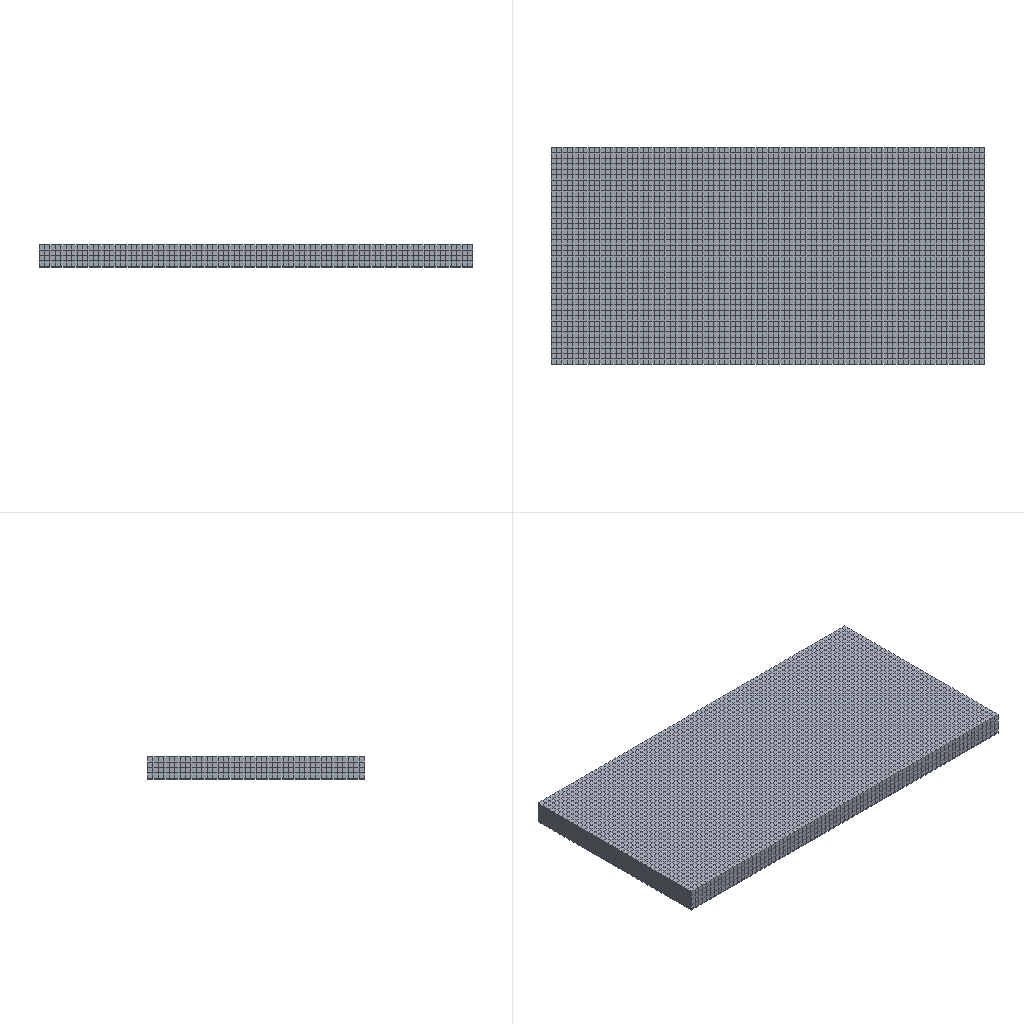Simulation study | abaqus
Set-up summary:
category,name,step,type,value,unit,region
solver,abaqus
solver,version,,,Abaqus/Explicit 2020
units,not stated in the deck,,not stated
analysis,deck,,transient,transient
load_step,Step-1,Step-1,transient
load_step,requested,,,1
mesh,nodes,,,23247
mesh,elements,,,19200
element_type,C3D8R,,solid,16000
element_type,COH3D8,,cohesive,3200
load,load commands in deck,,count,1
bc,support commands in deck,,count,1
material,BASE,,in results
material,COH,,in results
material,MO,,in results
check,setup vs results,,match,"per instance, exact: element labels, types and connectivity; labels of the nodes the elements use; coordinates of those nodes at SINGLE_PRECISION in 1 of 1 instance(s)"
Abaqus input file, long lists of numbers shortened:
*Heading
** Job name: Job-1 Model name: Model-1
** Generated by: Abaqus/CAE 2020
*Preprint, echo=NO, model=NO, history=NO, contact=NO
**
** PARTS
**
*Part, name=fianl
*Node
      1,         400.,           0.,          20.
      2,         400.,        -200.,          20.
** (23245 more lines like these left out)
*Element, type=C3D8R
    1,   338,  1441, 10684,   967,     1,    13,   733,    96
    2,  1441,  1442, 10685, 10684,    13,    14,   734,   733
** (15998 more lines like these left out)
*Element, type=COH3D8
16001,  4522,    93,     4,   181, 19930, 19929, 19928, 19927
16002,  4523,    92,    93,  4522, 19932, 19931, 19929, 19930
** (3198 more lines like these left out)
*Nset, nset=Set-1
     3,     4,     6,     7,     9,    10,    11,    12,    55,    56,    57,    58,    59,    60,    61,    62
    63,    64,    65,    66,    67,    68,    69,    70,    71,    72,    73,    74,    75,    76,    77,    78
** (414 more lines like these left out)
*Elset, elset=Set-1, generate
 12801,  16000,      1
*Nset, nset=Set-2
     1,     2,     5,     8,    13,    14,    15,    16,    17,    18,    19,    20,    21,    22,    23,    24
    25,    26,    27,    28,    29,    30,    31,    32,    33,    34,    35,    36,    37,    38,    39,    40
** (1036 more lines like these left out)
*Elset, elset=Set-2, generate
     1,  12800,      1
*Elset, elset=CohesiveSeam-1-Elements, generate
 16001,  19200,      1
*Nset, nset=CohesiveSeam-1-TopNodes, generate
 19927,  23247,      1
*Nset, nset=CohesiveSeam-1-BottomNodes
    3,    4,    6,    7,   55,   56,   57,   58,   59,   60,   61,   62,   63,   64,   65,   66
   67,   68,   69,   70,   71,   72,   73,   74,   75,   76,   77,   78,   79,   80,   81,   82
** (206 more lines like these left out)
*Elset, elset=__PickedSurf5_#2_S1, internal, generate
 16001,  19200,      1
*Surface, type=ELEMENT, name=_PickedSurf5_#2, internal
__PickedSurf5_#2_S1, S1
*Elset, elset=__PickedSurf7_S1, internal, generate
 16001,  19200,      1
*Surface, type=ELEMENT, name=_PickedSurf7, internal
__PickedSurf7_S1, S1
*Elset, elset=_CohesiveSeam-1-TopSurf_S2, internal, generate
 16001,  19200,      1
*Surface, type=ELEMENT, name=CohesiveSeam-1-TopSurf
_CohesiveSeam-1-TopSurf_S2, S2
*Elset, elset=_CohesiveSeam-1-BottomSurf_S1, internal, generate
 16001,  19200,      1
*Surface, type=ELEMENT, name=CohesiveSeam-1-BottomSurf
_CohesiveSeam-1-BottomSurf_S1, S1
** Section: Section-2
*Solid Section, elset=Set-2, material=base
,
** Section: Section-1
*Solid Section, elset=Set-1, material=mo
,
** Section: coh
*Cohesive Section, elset=CohesiveSeam-1-Elements, controls=EC-1, material=coh, response=TRACTION SEPARATION
,
*End Part
**
**
** ASSEMBLY
**
*Assembly, name=Assembly
**
*Instance, name=fianl-1, part=fianl
*End Instance
**
*Nset, nset=Set-1, instance=fianl-1, generate
     1,  23247,      1
*Elset, elset=Set-1, instance=fianl-1, generate
     1,  19200,      1
*Nset, nset=Set-2, instance=fianl-1
    1,    2,    5,    8,   13,   14,   15,   16,   17,   18,   19,   20,   21,   22,   23,   24
   25,   26,   27,   28,   29,   30,   31,   32,   33,   34,   35,   36,   37,   38,   39,   40
** (206 more lines like these left out)
*Elset, elset=Set-2, instance=fianl-1
     1,     2,     3,     4,     5,     6,     7,     8,     9,    10,    11,    12,    13,    14,    15,    16
    17,    18,    19,    20,    21,    22,    23,    24,    25,    26,    27,    28,    29,    30,    31,    32
** (198 more lines like these left out)
*Nset, nset=Set-3, instance=fianl-1
     3,     4,     6,     7,     9,    10,    11,    12,    55,    56,    57,    58,    59,    60,    61,    62
    63,    64,    65,    66,    67,    68,    69,    70,    71,    72,    73,    74,    75,    76,    77,    78
** (621 more lines like these left out)
*Elset, elset=Set-3, instance=fianl-1, generate
 12801,  19200,      1
*Nset, nset=Set-4, instance=fianl-1, generate
     1,  23247,      1
*Elset, elset=Set-4, instance=fianl-1, generate
     1,  19200,      1
*Nset, nset=Set-5, instance=fianl-1
     3,     4,     6,     7,     9,    10,    11,    12,    55,    56,    57,    58,    59,    60,    61,    62
    63,    64,    65,    66,    67,    68,    69,    70,    71,    72,    73,    74,    75,    76,    77,    78
** (414 more lines like these left out)
*Elset, elset=Set-5, instance=fianl-1, generate
 12801,  16000,      1
*Nset, nset=Set-6, instance=fianl-1
    1,    2,    5,    8,   13,   14,   15,   16,   17,   18,   19,   20,   21,   22,   23,   24
   25,   26,   27,   28,   29,   30,   31,   32,   33,   34,   35,   36,   37,   38,   39,   40
** (206 more lines like these left out)
*Elset, elset=Set-6, instance=fianl-1
     1,     2,     3,     4,     5,     6,     7,     8,     9,    10,    11,    12,    13,    14,    15,    16
    17,    18,    19,    20,    21,    22,    23,    24,    25,    26,    27,    28,    29,    30,    31,    32
** (198 more lines like these left out)
*Nset, nset=Set-7, instance=fianl-1
   3,   4,   6,   7,   9,  10,  11,  12, 181, 182, 183, 184, 185, 186, 187, 188
 189, 190, 191, 192, 193, 194, 195, 196, 197, 198, 199, 200, 201, 202, 203, 204
** (19 more lines like these left out)
*Elset, elset=Set-7, instance=fianl-1
 12801, 12840, 12841, 12880, 12881, 12920, 12921, 12960, 12961, 13000, 13001, 13040, 13041, 13080, 13081, 13120
 13121, 13160, 13161, 13200, 13201, 13240, 13241, 13280, 13281, 13320, 13321, 13360, 13361, 13400, 13401, 13440
** (8 more lines like these left out)
*Nset, nset=Set-8, instance=fianl-1
   3,   4,   6,   7,   9,  10,  11,  12,  55,  56,  57,  58,  59,  60,  61,  62
  63,  64,  65,  66,  67,  68,  69,  70,  71,  72,  73,  74,  75,  76,  77,  78
** (9 more lines like these left out)
*Elset, elset=Set-8, instance=fianl-1
 12801, 12802, 12803, 12804, 12805, 12806, 12807, 12808, 12809, 12810, 12811, 12812, 12813, 12814, 12815, 12816
 12817, 12818, 12819, 12820, 12821, 12822, 12823, 12824, 12825, 12826, 12827, 12828, 12829, 12830, 12831, 12832
** (3 more lines like these left out)
*End Assembly
**
** ELEMENT CONTROLS
**
*Section Controls, name=EC-1, ELEMENT DELETION=YES
1., 1., 1.
**
** MATERIALS
**
*Material, name=base
*Density
 3e-09,
*Elastic
80000., 0.22
*Material, name=coh
*Damage Initiation, criterion=MAXS
 0.01, 0.05, 0.03
*Damage Evolution, type=DISPLACEMENT
 1e-12,
*Density
 1e-09,
*Elastic, type=TRACTION
10.,10.,10.
*Expansion
 0.01,
*Material, name=mo
*Density
 1e-09,
*Elastic
1., 0.45
*Expansion
 5e-05,
*Plastic
167.,0.
**
** PREDEFINED FIELDS
**
** Name: Predefined Field-1   Type: Temperature
*Initial Conditions, type=TEMPERATURE
Set-4, 20.
** ----------------------------------------------------------------
**
** STEP: Step-1
**
*Step, name=Step-1, nlgeom=YES
*Dynamic, Explicit
, 0.01
*Bulk Viscosity
0.06, 1.2
**
** BOUNDARY CONDITIONS
**
** Name: BC-1 Type: 对称/反对称/完全固定
*Boundary
Set-6, ENCASTRE
**
** PREDEFINED FIELDS
**
** Name: Predefined Field-2   Type: Temperature
*Temperature
Set-5, 800.
**
** OUTPUT REQUESTS
**
*Restart, write, number interval=1, time marks=NO
**
** FIELD OUTPUT: F-Output-1
**
*Output, field
*Node Output
A, CF, RF, RM, RT, U, V
*Element Output, directions=YES
E, LE, MISES, MISESONLY, PE, PEEQ, PEEQMAX, PEEQT, PEEQVAVG, PEMAG, PEVAVG, PRESSONLY, S, SDEG, SF, SSAVG
STATUS, SVAVG, TEMP, YIELDPOT
*Contact Output
CDISP, CSDMG, CSTRESS
**
** HISTORY OUTPUT: H-Output-1
**
*Output, history, variable=PRESELECT
*End Step
Results summary:
result,step,Step-1,completed,increments=12745 time=0.01/0.01
result,analysis,,,transient
result,last_loadstep,,,1
result,primary field,,,U
result,reaction total,,FX,2e-06,model units
result,reaction total,,FY,1.5e-05,model units
result,reaction total,,FZ,-1.376,model units